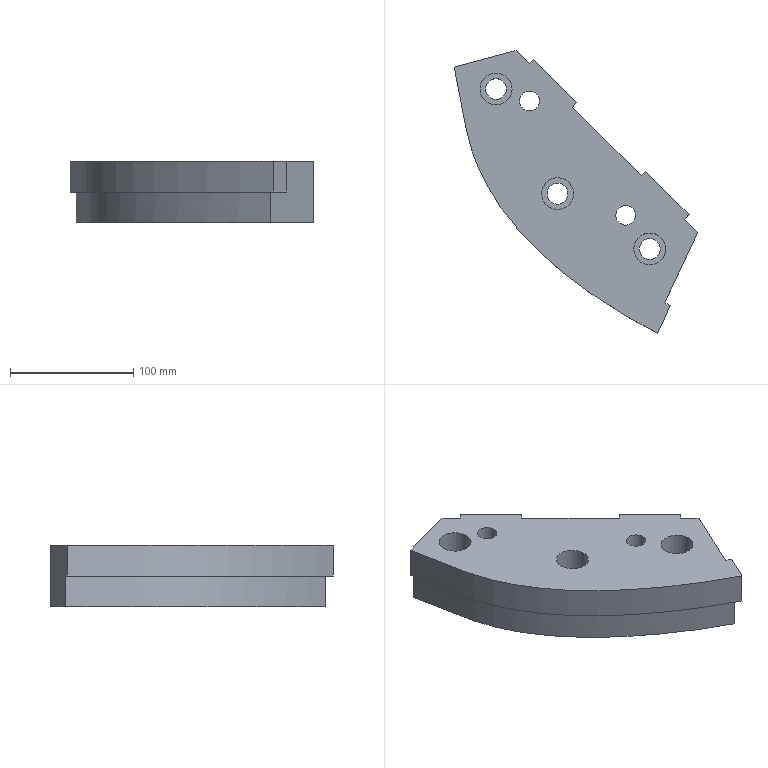Part | NX | features solid 2 | 1 solid | 29 faces | box 197.946 x 229.951 x 50 mm | volume 1003204 mm3 | plane 19 | cylinder 8 | spline 2 | commonest cylinder face diameters 17 x3 26 x3 16 x2
STEP:
#1=CARTESIAN_POINT('',(-617.89,-159.555,-25.));
#2=VERTEX_POINT('',#1);
#3=CARTESIAN_POINT('',(-609.536,-141.638,-25.));
#4=VERTEX_POINT('',#3);
#5=CARTESIAN_POINT('',(-620.101,-164.296,-25.));
#6=DIRECTION('',(-0.4226,-0.9063,0.));
#7=VECTOR('',#6,1000.);
#8=LINE('',#5,#7);
#9=EDGE_CURVE('',#2,#4,#8,.F.);
#10=ORIENTED_EDGE('',*,*,#9,.T.);
#11=CARTESIAN_POINT('',(-605.004,-143.752,-25.));
#12=VERTEX_POINT('',#11);
#13=CARTESIAN_POINT('',(-609.536,-141.638,-25.));
#14=DIRECTION('',(0.9063,-0.4226,0.));
#15=VECTOR('',#14,1000.);
#16=LINE('',#13,#15);
#17=EDGE_CURVE('',#4,#12,#16,.T.);
#18=ORIENTED_EDGE('',*,*,#17,.T.);
#19=CARTESIAN_POINT('',(-615.57,-166.409,-25.));
#20=VERTEX_POINT('',#19);
#21=CARTESIAN_POINT('',(-615.57,-166.409,-25.));
#22=DIRECTION('',(-0.4226,-0.9063,0.));
#23=VECTOR('',#22,1000.);
#24=LINE('',#21,#23);
#25=EDGE_CURVE('',#12,#20,#24,.T.);
#26=ORIENTED_EDGE('',*,*,#25,.T.);
#27=CARTESIAN_POINT('',(-780.695,50.088,-25.));
#28=VERTEX_POINT('',#27);
#29=CARTESIAN_POINT('',(-780.695,50.088,-25.));
#30=CARTESIAN_POINT('',(-778.803,40.269,-25.));
#31=CARTESIAN_POINT('',(-776.28,27.176,-25.));
#32=CARTESIAN_POINT('',(-773.127,10.811,-25.));
#33=CARTESIAN_POINT('',(-771.556,2.503,-25.));
#34=CARTESIAN_POINT('',(-770.053,-4.764,-25.));
#35=CARTESIAN_POINT('',(-768.05,-12.691,-25.));
#36=CARTESIAN_POINT('',(-763.621,-26.574,-25.));
#37=CARTESIAN_POINT('',(-751.782,-52.713,-25.));
#38=CARTESIAN_POINT('',(-727.402,-85.879,-25.));
#39=CARTESIAN_POINT('',(-691.163,-119.147,-25.));
#40=CARTESIAN_POINT('',(-653.334,-145.582,-25.));
#41=CARTESIAN_POINT('',(-627.462,-160.273,-25.));
#42=CARTESIAN_POINT('',(-615.57,-166.409,-25.));
#43=B_SPLINE_CURVE_WITH_KNOTS('',3,(#29,#30,#31,#32,#33,#34,#35,#36,#37,#38,#39,#40,#41,#42),.UNSPECIFIED.,.F.,.F.,(4,1,1,1,1,1,1,1,1,1,1,4),(0.,0.1048,0.1397,0.1746,0.1934,0.2175,0.2603,0.3459,0.5172,0.6885,0.8598,1.),.UNSPECIFIED.);
#44=EDGE_CURVE('',#20,#28,#43,.F.);
#45=ORIENTED_EDGE('',*,*,#44,.T.);
#46=CARTESIAN_POINT('',(-775.853,51.386,-25.));
#47=VERTEX_POINT('',#46);
#48=CARTESIAN_POINT('',(-780.695,50.088,-25.));
#49=DIRECTION('',(-0.9659,-0.2588,0.));
#50=VECTOR('',#49,1000.);
#51=LINE('',#48,#50);
#52=EDGE_CURVE('',#47,#28,#51,.T.);
#53=ORIENTED_EDGE('',*,*,#52,.F.);
#54=CARTESIAN_POINT('',(-775.853,51.386,-25.));
#55=CARTESIAN_POINT('',(-774.744,45.629,-25.));
#56=CARTESIAN_POINT('',(-772.527,34.112,-25.));
#57=CARTESIAN_POINT('',(-769.748,19.729,-25.));
#58=CARTESIAN_POINT('',(-767.541,8.189,-25.));
#59=CARTESIAN_POINT('',(-765.905,-0.4077,-25.));
#60=CARTESIAN_POINT('',(-763.978,-8.633,-25.));
#61=CARTESIAN_POINT('',(-760.703,-19.53,-25.));
#62=CARTESIAN_POINT('',(-755.498,-32.754,-25.));
#63=CARTESIAN_POINT('',(-744.953,-52.969,-25.));
#64=CARTESIAN_POINT('',(-728.152,-76.258,-25.));
#65=CARTESIAN_POINT('',(-703.994,-101.032,-25.));
#66=CARTESIAN_POINT('',(-668.1,-130.302,-25.));
#67=CARTESIAN_POINT('',(-638.408,-148.692,-25.));
#68=CARTESIAN_POINT('',(-617.89,-159.555,-25.));
#69=B_SPLINE_CURVE_WITH_KNOTS('',3,(#54,#55,#56,#57,#58,#59,#60,#61,#62,#63,#64,#65,#66,#67,#68),.UNSPECIFIED.,.F.,.F.,(4,1,1,1,1,1,1,1,1,1,1,1,4),(-0.00125,0.06018,0.1216,0.1523,0.183,0.2138,0.2445,0.3059,0.3673,0.4902,0.6131,0.7359,0.9816),.UNSPECIFIED.);
#70=EDGE_CURVE('',#47,#2,#69,.T.);
#71=ORIENTED_EDGE('',*,*,#70,.T.);
#72=EDGE_LOOP('',(#10,#18,#26,#45,#53,#71));
#73=FACE_BOUND('',#72,.T.);
#74=CARTESIAN_POINT('',(-615.57,-166.409,-25.));
#75=DIRECTION('',(0.,0.,-1.));
#76=DIRECTION('',(-1.,0.,0.));
#77=AXIS2_PLACEMENT_3D('',#74,#75,#76);
#78=PLANE('',#77);
#79=ADVANCED_FACE('',(#73),#78,.T.);
#80=CARTESIAN_POINT('',(-727.523,22.579,0.));
#81=VERTEX_POINT('',#80);
#82=CARTESIAN_POINT('',(-719.523,22.579,0.));
#83=DIRECTION('',(0.,0.,-1.));
#84=DIRECTION('',(-1.,0.,0.));
#85=AXIS2_PLACEMENT_3D('',#82,#83,#84);
#86=CIRCLE('',#85,8.);
#87=EDGE_CURVE('',#81,#81,#86,.T.);
#88=ORIENTED_EDGE('',*,*,#87,.T.);
#89=EDGE_LOOP('',(#88));
#90=FACE_BOUND('',#89,.T.);
#91=CARTESIAN_POINT('',(-649.374,-70.368,0.));
#92=VERTEX_POINT('',#91);
#93=CARTESIAN_POINT('',(-641.374,-70.368,0.));
#94=DIRECTION('',(0.,0.,-1.));
#95=DIRECTION('',(-1.,0.,0.));
#96=AXIS2_PLACEMENT_3D('',#93,#94,#95);
#97=CIRCLE('',#96,8.);
#98=EDGE_CURVE('',#92,#92,#97,.T.);
#99=ORIENTED_EDGE('',*,*,#98,.T.);
#100=EDGE_LOOP('',(#99));
#101=FACE_BOUND('',#100,.T.);
#102=CARTESIAN_POINT('',(-683.729,-52.741,0.));
#103=VERTEX_POINT('',#102);
#104=CARTESIAN_POINT('',(-696.729,-52.741,0.));
#105=DIRECTION('',(0.,0.,1.));
#106=DIRECTION('',(1.,0.,0.));
#107=AXIS2_PLACEMENT_3D('',#104,#105,#106);
#108=CIRCLE('',#107,13.);
#109=EDGE_CURVE('',#103,#103,#108,.T.);
#110=ORIENTED_EDGE('',*,*,#109,.F.);
#111=EDGE_LOOP('',(#110));
#112=FACE_BOUND('',#111,.T.);
#113=CARTESIAN_POINT('',(-608.729,-97.741,0.));
#114=VERTEX_POINT('',#113);
#115=CARTESIAN_POINT('',(-621.729,-97.741,0.));
#116=DIRECTION('',(0.,0.,1.));
#117=DIRECTION('',(1.,0.,0.));
#118=AXIS2_PLACEMENT_3D('',#115,#116,#117);
#119=CIRCLE('',#118,13.);
#120=EDGE_CURVE('',#114,#114,#119,.T.);
#121=ORIENTED_EDGE('',*,*,#120,.F.);
#122=EDGE_LOOP('',(#121));
#123=FACE_BOUND('',#122,.T.);
#124=CARTESIAN_POINT('',(-733.729,32.259,0.));
#125=VERTEX_POINT('',#124);
#126=CARTESIAN_POINT('',(-746.729,32.259,0.));
#127=DIRECTION('',(0.,0.,1.));
#128=DIRECTION('',(1.,0.,0.));
#129=AXIS2_PLACEMENT_3D('',#126,#127,#128);
#130=CIRCLE('',#129,13.);
#131=EDGE_CURVE('',#125,#125,#130,.T.);
#132=ORIENTED_EDGE('',*,*,#131,.F.);
#133=EDGE_LOOP('',(#132));
#134=FACE_BOUND('',#133,.T.);
#135=CARTESIAN_POINT('',(-609.536,-141.638,0.));
#136=VERTEX_POINT('',#135);
#137=CARTESIAN_POINT('',(-605.004,-143.752,0.));
#138=VERTEX_POINT('',#137);
#139=CARTESIAN_POINT('',(-609.536,-141.638,0.));
#140=DIRECTION('',(0.9063,-0.4226,0.));
#141=VECTOR('',#140,1000.);
#142=LINE('',#139,#141);
#143=EDGE_CURVE('',#136,#138,#142,.T.);
#144=ORIENTED_EDGE('',*,*,#143,.F.);
#145=CARTESIAN_POINT('',(-582.749,-84.195,0.));
#146=VERTEX_POINT('',#145);
#147=CARTESIAN_POINT('',(-620.101,-164.296,0.));
#148=DIRECTION('',(0.4226,0.9063,0.));
#149=VECTOR('',#148,1000.);
#150=LINE('',#147,#149);
#151=EDGE_CURVE('',#136,#146,#150,.T.);
#152=ORIENTED_EDGE('',*,*,#151,.T.);
#153=CARTESIAN_POINT('',(-593.356,-73.588,0.));
#154=VERTEX_POINT('',#153);
#155=CARTESIAN_POINT('',(-730.486,63.542,0.));
#156=DIRECTION('',(0.7071,-0.7071,0.));
#157=VECTOR('',#156,1000.);
#158=LINE('',#155,#157);
#159=EDGE_CURVE('',#154,#146,#158,.T.);
#160=ORIENTED_EDGE('',*,*,#159,.F.);
#161=CARTESIAN_POINT('',(-589.82,-70.052,0.));
#162=VERTEX_POINT('',#161);
#163=CARTESIAN_POINT('',(-593.356,-73.588,0.));
#164=DIRECTION('',(0.7071,0.7071,0.));
#165=VECTOR('',#164,1000.);
#166=LINE('',#163,#165);
#167=EDGE_CURVE('',#154,#162,#166,.T.);
#168=ORIENTED_EDGE('',*,*,#167,.T.);
#169=CARTESIAN_POINT('',(-625.176,-34.697,0.));
#170=VERTEX_POINT('',#169);
#171=CARTESIAN_POINT('',(-726.95,67.077,0.));
#172=DIRECTION('',(0.7071,-0.7071,0.));
#173=VECTOR('',#172,1000.);
#174=LINE('',#171,#173);
#175=EDGE_CURVE('',#170,#162,#174,.T.);
#176=ORIENTED_EDGE('',*,*,#175,.F.);
#177=CARTESIAN_POINT('',(-628.711,-38.233,0.));
#178=VERTEX_POINT('',#177);
#179=CARTESIAN_POINT('',(-628.711,-38.233,0.));
#180=DIRECTION('',(0.7071,0.7071,0.));
#181=VECTOR('',#180,1000.);
#182=LINE('',#179,#181);
#183=EDGE_CURVE('',#178,#170,#182,.T.);
#184=ORIENTED_EDGE('',*,*,#183,.F.);
#185=CARTESIAN_POINT('',(-684.524,17.58,0.));
#186=VERTEX_POINT('',#185);
#187=CARTESIAN_POINT('',(-730.486,63.542,0.));
#188=DIRECTION('',(0.7071,-0.7071,0.));
#189=VECTOR('',#188,1000.);
#190=LINE('',#187,#189);
#191=EDGE_CURVE('',#186,#178,#190,.T.);
#192=ORIENTED_EDGE('',*,*,#191,.F.);
#193=CARTESIAN_POINT('',(-680.988,21.115,0.));
#194=VERTEX_POINT('',#193);
#195=CARTESIAN_POINT('',(-684.524,17.58,0.));
#196=DIRECTION('',(0.7071,0.7071,0.));
#197=VECTOR('',#196,1000.);
#198=LINE('',#195,#197);
#199=EDGE_CURVE('',#186,#194,#198,.T.);
#200=ORIENTED_EDGE('',*,*,#199,.T.);
#201=CARTESIAN_POINT('',(-716.343,56.471,0.));
#202=VERTEX_POINT('',#201);
#203=CARTESIAN_POINT('',(-828.725,168.852,0.));
#204=DIRECTION('',(0.7071,-0.7071,0.));
#205=VECTOR('',#204,1000.);
#206=LINE('',#203,#205);
#207=EDGE_CURVE('',#202,#194,#206,.T.);
#208=ORIENTED_EDGE('',*,*,#207,.F.);
#209=CARTESIAN_POINT('',(-719.879,52.935,0.));
#210=VERTEX_POINT('',#209);
#211=CARTESIAN_POINT('',(-719.879,52.935,0.));
#212=DIRECTION('',(0.7071,0.7071,0.));
#213=VECTOR('',#212,1000.);
#214=LINE('',#211,#213);
#215=EDGE_CURVE('',#210,#202,#214,.T.);
#216=ORIENTED_EDGE('',*,*,#215,.F.);
#217=CARTESIAN_POINT('',(-730.486,63.542,0.));
#218=VERTEX_POINT('',#217);
#219=CARTESIAN_POINT('',(-730.486,63.542,0.));
#220=DIRECTION('',(0.7071,-0.7071,0.));
#221=VECTOR('',#220,1000.);
#222=LINE('',#219,#221);
#223=EDGE_CURVE('',#218,#210,#222,.T.);
#224=ORIENTED_EDGE('',*,*,#223,.F.);
#225=CARTESIAN_POINT('',(-780.695,50.088,0.));
#226=VERTEX_POINT('',#225);
#227=CARTESIAN_POINT('',(-780.695,50.088,0.));
#228=DIRECTION('',(0.9659,0.2588,0.));
#229=VECTOR('',#228,1000.);
#230=LINE('',#227,#229);
#231=EDGE_CURVE('',#226,#218,#230,.T.);
#232=ORIENTED_EDGE('',*,*,#231,.F.);
#233=CARTESIAN_POINT('',(-615.57,-166.409,0.));
#234=VERTEX_POINT('',#233);
#235=CARTESIAN_POINT('',(-780.695,50.088,0.));
#236=CARTESIAN_POINT('',(-778.803,40.269,0.));
#237=CARTESIAN_POINT('',(-776.28,27.176,0.));
#238=CARTESIAN_POINT('',(-773.127,10.811,0.));
#239=CARTESIAN_POINT('',(-771.556,2.503,0.));
#240=CARTESIAN_POINT('',(-770.053,-4.764,0.));
#241=CARTESIAN_POINT('',(-768.05,-12.691,0.));
#242=CARTESIAN_POINT('',(-763.621,-26.574,0.));
#243=CARTESIAN_POINT('',(-751.782,-52.713,0.));
#244=CARTESIAN_POINT('',(-727.402,-85.879,0.));
#245=CARTESIAN_POINT('',(-691.163,-119.147,0.));
#246=CARTESIAN_POINT('',(-653.334,-145.582,0.));
#247=CARTESIAN_POINT('',(-627.462,-160.273,0.));
#248=CARTESIAN_POINT('',(-615.57,-166.409,0.));
#249=B_SPLINE_CURVE_WITH_KNOTS('',3,(#235,#236,#237,#238,#239,#240,#241,#242,#243,#244,#245,#246,#247,#248),.UNSPECIFIED.,.F.,.F.,(4,1,1,1,1,1,1,1,1,1,1,4),(0.,0.1048,0.1397,0.1746,0.1934,0.2175,0.2603,0.3459,0.5172,0.6885,0.8598,1.),.UNSPECIFIED.);
#250=EDGE_CURVE('',#226,#234,#249,.T.);
#251=ORIENTED_EDGE('',*,*,#250,.T.);
#252=CARTESIAN_POINT('',(-615.57,-166.409,0.));
#253=DIRECTION('',(0.4226,0.9063,0.));
#254=VECTOR('',#253,1000.);
#255=LINE('',#252,#254);
#256=EDGE_CURVE('',#234,#138,#255,.T.);
#257=ORIENTED_EDGE('',*,*,#256,.T.);
#258=EDGE_LOOP('',(#144,#152,#160,#168,#176,#184,#192,#200,#208,#216,#224,#232,#251,#257));
#259=FACE_BOUND('',#258,.T.);
#260=CARTESIAN_POINT('',(-733.42,73.248,0.));
#261=DIRECTION('',(0.,0.,-1.));
#262=DIRECTION('',(-1.,0.,0.));
#263=AXIS2_PLACEMENT_3D('',#260,#261,#262);
#264=PLANE('',#263);
#265=ADVANCED_FACE('',(#90,#101,#112,#123,#134,#259),#264,.F.);
#266=ORIENTED_EDGE('',*,*,#25,.F.);
#267=CARTESIAN_POINT('',(-605.004,-143.752,-50.));
#268=DIRECTION('',(0.,0.,1.));
#269=VECTOR('',#268,1000.);
#270=LINE('',#267,#269);
#271=EDGE_CURVE('',#12,#138,#270,.T.);
#272=ORIENTED_EDGE('',*,*,#271,.T.);
#273=ORIENTED_EDGE('',*,*,#256,.F.);
#274=CARTESIAN_POINT('',(-615.57,-166.409,-70.));
#275=DIRECTION('',(0.,0.,1.));
#276=VECTOR('',#275,1000.);
#277=LINE('',#274,#276);
#278=EDGE_CURVE('',#20,#234,#277,.T.);
#279=ORIENTED_EDGE('',*,*,#278,.F.);
#280=EDGE_LOOP('',(#266,#272,#273,#279));
#281=FACE_BOUND('',#280,.T.);
#282=CARTESIAN_POINT('',(-615.57,-166.409,-50.));
#283=DIRECTION('',(0.9063,-0.4226,0.));
#284=DIRECTION('',(0.4226,0.9063,0.));
#285=AXIS2_PLACEMENT_3D('',#282,#283,#284);
#286=PLANE('',#285);
#287=ADVANCED_FACE('',(#281),#286,.T.);
#288=ORIENTED_EDGE('',*,*,#159,.T.);
#289=CARTESIAN_POINT('',(-582.749,-84.195,-50.));
#290=VERTEX_POINT('',#289);
#291=CARTESIAN_POINT('',(-582.749,-84.195,-50.));
#292=DIRECTION('',(0.,0.,-1.));
#293=VECTOR('',#292,1000.);
#294=LINE('',#291,#293);
#295=EDGE_CURVE('',#146,#290,#294,.T.);
#296=ORIENTED_EDGE('',*,*,#295,.T.);
#297=CARTESIAN_POINT('',(-593.356,-73.588,-50.));
#298=VERTEX_POINT('',#297);
#299=CARTESIAN_POINT('',(-730.486,63.542,-50.));
#300=DIRECTION('',(0.7071,-0.7071,0.));
#301=VECTOR('',#300,1000.);
#302=LINE('',#299,#301);
#303=EDGE_CURVE('',#298,#290,#302,.T.);
#304=ORIENTED_EDGE('',*,*,#303,.F.);
#305=CARTESIAN_POINT('',(-593.356,-73.588,-50.));
#306=DIRECTION('',(0.,0.,1.));
#307=VECTOR('',#306,1000.);
#308=LINE('',#305,#307);
#309=EDGE_CURVE('',#298,#154,#308,.T.);
#310=ORIENTED_EDGE('',*,*,#309,.T.);
#311=EDGE_LOOP('',(#288,#296,#304,#310));
#312=FACE_BOUND('',#311,.T.);
#313=CARTESIAN_POINT('',(-730.486,63.542,-50.));
#314=DIRECTION('',(-0.7071,-0.7071,0.));
#315=DIRECTION('',(0.7071,-0.7071,0.));
#316=AXIS2_PLACEMENT_3D('',#313,#314,#315);
#317=PLANE('',#316);
#318=ADVANCED_FACE('',(#312),#317,.F.);
#319=CARTESIAN_POINT('',(-711.523,22.579,-50.));
#320=VERTEX_POINT('',#319);
#321=CARTESIAN_POINT('',(-719.523,22.579,-50.));
#322=DIRECTION('',(0.,0.,1.));
#323=DIRECTION('',(1.,0.,0.));
#324=AXIS2_PLACEMENT_3D('',#321,#322,#323);
#325=CIRCLE('',#324,8.);
#326=EDGE_CURVE('',#320,#320,#325,.T.);
#327=ORIENTED_EDGE('',*,*,#326,.T.);
#328=EDGE_LOOP('',(#327));
#329=FACE_BOUND('',#328,.T.);
#330=CARTESIAN_POINT('',(-633.374,-70.368,-50.));
#331=VERTEX_POINT('',#330);
#332=CARTESIAN_POINT('',(-641.374,-70.368,-50.));
#333=DIRECTION('',(0.,0.,1.));
#334=DIRECTION('',(1.,0.,0.));
#335=AXIS2_PLACEMENT_3D('',#332,#333,#334);
#336=CIRCLE('',#335,8.);
#337=EDGE_CURVE('',#331,#331,#336,.T.);
#338=ORIENTED_EDGE('',*,*,#337,.T.);
#339=EDGE_LOOP('',(#338));
#340=FACE_BOUND('',#339,.T.);
#341=CARTESIAN_POINT('',(-617.89,-159.555,-50.));
#342=VERTEX_POINT('',#341);
#343=CARTESIAN_POINT('',(-607.768,-137.848,-50.));
#344=DIRECTION('',(-0.4226,-0.9063,0.));
#345=VECTOR('',#344,1000.);
#346=LINE('',#343,#345);
#347=EDGE_CURVE('',#290,#342,#346,.T.);
#348=ORIENTED_EDGE('',*,*,#347,.T.);
#349=CARTESIAN_POINT('',(-775.853,51.386,-50.));
#350=VERTEX_POINT('',#349);
#351=CARTESIAN_POINT('',(-617.89,-159.555,-50.));
#352=CARTESIAN_POINT('',(-622.998,-156.85,-50.));
#353=CARTESIAN_POINT('',(-630.561,-152.674,-50.));
#354=CARTESIAN_POINT('',(-639.19,-147.603,-50.));
#355=CARTESIAN_POINT('',(-644.088,-144.635,-50.));
#356=CARTESIAN_POINT('',(-647.684,-142.412,-50.));
#357=CARTESIAN_POINT('',(-651.449,-140.037,-50.));
#358=CARTESIAN_POINT('',(-656.324,-136.895,-50.));
#359=CARTESIAN_POINT('',(-662.31,-132.912,-50.));
#360=CARTESIAN_POINT('',(-668.126,-128.871,-50.));
#361=CARTESIAN_POINT('',(-672.085,-126.03,-50.));
#362=CARTESIAN_POINT('',(-674.358,-124.372,-50.));
#363=CARTESIAN_POINT('',(-675.947,-123.2,-50.));
#364=CARTESIAN_POINT('',(-677.912,-121.734,-50.));
#365=CARTESIAN_POINT('',(-680.368,-119.877,-50.));
#366=CARTESIAN_POINT('',(-683.437,-117.514,-50.));
#367=CARTESIAN_POINT('',(-687.023,-114.68,-50.));
#368=CARTESIAN_POINT('',(-691.708,-110.88,-50.));
#369=CARTESIAN_POINT('',(-697.371,-106.101,-50.));
#370=CARTESIAN_POINT('',(-703.86,-100.315,-50.));
#371=CARTESIAN_POINT('',(-710.042,-94.48,-50.));
#372=CARTESIAN_POINT('',(-714.937,-89.576,-50.));
#373=CARTESIAN_POINT('',(-718.7,-85.627,-50.));
#374=CARTESIAN_POINT('',(-721.444,-82.656,-50.));
#375=CARTESIAN_POINT('',(-723.673,-80.162,-50.));
#376=CARTESIAN_POINT('',(-725.186,-78.425,-50.));
#377=CARTESIAN_POINT('',(-726.062,-77.408,-50.));
#378=CARTESIAN_POINT('',(-726.657,-76.711,-50.));
#379=CARTESIAN_POINT('',(-727.462,-75.759,-50.));
#380=CARTESIAN_POINT('',(-728.451,-74.577,-50.));
#381=CARTESIAN_POINT('',(-730.192,-72.464,-50.));
#382=CARTESIAN_POINT('',(-732.591,-69.456,-50.));
#383=CARTESIAN_POINT('',(-735.368,-65.82,-50.));
#384=CARTESIAN_POINT('',(-738.921,-60.952,-50.));
#385=CARTESIAN_POINT('',(-743.087,-54.822,-50.));
#386=CARTESIAN_POINT('',(-749.161,-44.924,-50.));
#387=CARTESIAN_POINT('',(-754.356,-34.877,-50.));
#388=CARTESIAN_POINT('',(-758.119,-25.991,-50.));
#389=CARTESIAN_POINT('',(-760.062,-20.837,-50.));
#390=CARTESIAN_POINT('',(-761.372,-17.07,-50.));
#391=CARTESIAN_POINT('',(-762.709,-12.844,-50.));
#392=CARTESIAN_POINT('',(-763.892,-8.672,-50.));
#393=CARTESIAN_POINT('',(-764.791,-5.118,-50.));
#394=CARTESIAN_POINT('',(-765.365,-2.621,-50.));
#395=CARTESIAN_POINT('',(-765.643,-1.351,-50.));
#396=CARTESIAN_POINT('',(-765.793,-0.6486,-50.));
#397=CARTESIAN_POINT('',(-765.918,-0.04992,-50.));
#398=CARTESIAN_POINT('',(-765.986,0.2783,-50.));
#399=CARTESIAN_POINT('',(-766.102,0.8432,-50.));
#400=CARTESIAN_POINT('',(-766.307,1.853,-50.));
#401=CARTESIAN_POINT('',(-766.637,3.514,-50.));
#402=CARTESIAN_POINT('',(-767.013,5.436,-50.));
#403=CARTESIAN_POINT('',(-767.295,6.9,-50.));
#404=CARTESIAN_POINT('',(-767.469,7.808,-50.));
#405=CARTESIAN_POINT('',(-767.586,8.417,-50.));
#406=CARTESIAN_POINT('',(-767.772,9.392,-50.));
#407=CARTESIAN_POINT('',(-767.982,10.486,-50.));
#408=CARTESIAN_POINT('',(-768.23,11.784,-50.));
#409=CARTESIAN_POINT('',(-768.488,13.135,-50.));
#410=CARTESIAN_POINT('',(-768.786,14.69,-50.));
#411=CARTESIAN_POINT('',(-769.014,15.883,-50.));
#412=CARTESIAN_POINT('',(-769.162,16.657,-50.));
#413=CARTESIAN_POINT('',(-769.244,17.082,-50.));
#414=CARTESIAN_POINT('',(-769.249,17.106,-50.));
#415=CARTESIAN_POINT('',(-769.269,17.211,-50.));
#416=CARTESIAN_POINT('',(-769.309,17.421,-50.));
#417=CARTESIAN_POINT('',(-769.399,17.887,-50.));
#418=CARTESIAN_POINT('',(-769.553,18.686,-50.));
#419=CARTESIAN_POINT('',(-769.821,20.079,-50.));
#420=CARTESIAN_POINT('',(-770.274,22.431,-50.));
#421=CARTESIAN_POINT('',(-771.007,26.232,-50.));
#422=CARTESIAN_POINT('',(-771.927,31.012,-50.));
#423=CARTESIAN_POINT('',(-773.407,38.69,-50.));
#424=CARTESIAN_POINT('',(-774.799,45.916,-50.));
#425=CARTESIAN_POINT('',(-775.853,51.386,-50.));
#426=B_SPLINE_CURVE_WITH_KNOTS('',3,(#351,#352,#353,#354,#355,#356,#357,#358,#359,#360,#361,#362,#363,#364,#365,#366,#367,#368,#369,#370,#371,#372,#373,#374,#375,#376,#377,#378,#379,#380,#381,#382,#383,#384,#385,#386,#387,#388,#389,#390,#391,#392,#393,#394,#395,#396,#397,#398,#399,#400,#401,#402,#403,#404,#405,#406,#407,#408,#409,#410,#411,#412,#413,#414,#415,#416,#417,#418,#419,#420,#421,#422,#423,#424,#425),.UNSPECIFIED.,.F.,.F.,(4,1,1,1,1,1,1,1,1,1,1,1,1,1,1,1,1,1,1,1,1,1,1,1,1,1,1,1,1,1,1,1,1,1,1,1,1,1,1,1,1,1,1,1,1,1,1,1,1,1,1,1,1,1,1,1,1,1,1,1,1,1,1,1,1,1,1,1,1,1,1,1,4),(0.,0.0625,0.09375,0.1094,0.125,0.1406,0.1562,0.1875,0.2188,0.2344,0.2422,0.25,0.2578,0.2656,0.2812,0.2969,0.3125,0.3438,0.375,0.4062,0.4375,0.4531,0.4688,0.4844,0.4922,0.4961,0.5,0.5039,0.5078,0.5156,0.5312,0.5469,0.5625,0.5938,0.625,0.6875,0.7188,0.7344,0.75,0.7656,0.7812,0.7969,0.8047,0.8086,0.8105,0.8125,0.8145,0.8164,0.8203,0.8281,0.8359,0.8398,0.8418,0.8438,0.8457,0.8477,0.8516,0.8555,0.8594,0.8672,0.8711,0.875,0.877,0.8789,0.8828,0.8906,0.8984,0.9062,0.9219,0.9375,0.9531,0.9688,1.),.UNSPECIFIED.);
#427=EDGE_CURVE('',#342,#350,#426,.T.);
#428=ORIENTED_EDGE('',*,*,#427,.T.);
#429=CARTESIAN_POINT('',(-730.486,63.542,-50.));
#430=VERTEX_POINT('',#429);
#431=CARTESIAN_POINT('',(-780.695,50.088,-50.));
#432=DIRECTION('',(0.9659,0.2588,0.));
#433=VECTOR('',#432,1000.);
#434=LINE('',#431,#433);
#435=EDGE_CURVE('',#350,#430,#434,.T.);
#436=ORIENTED_EDGE('',*,*,#435,.T.);
#437=CARTESIAN_POINT('',(-719.879,52.935,-50.));
#438=VERTEX_POINT('',#437);
#439=CARTESIAN_POINT('',(-730.486,63.542,-50.));
#440=DIRECTION('',(0.7071,-0.7071,0.));
#441=VECTOR('',#440,1000.);
#442=LINE('',#439,#441);
#443=EDGE_CURVE('',#430,#438,#442,.T.);
#444=ORIENTED_EDGE('',*,*,#443,.T.);
#445=CARTESIAN_POINT('',(-716.343,56.471,-50.));
#446=VERTEX_POINT('',#445);
#447=CARTESIAN_POINT('',(-719.879,52.935,-50.));
#448=DIRECTION('',(0.7071,0.7071,0.));
#449=VECTOR('',#448,1000.);
#450=LINE('',#447,#449);
#451=EDGE_CURVE('',#438,#446,#450,.T.);
#452=ORIENTED_EDGE('',*,*,#451,.T.);
#453=CARTESIAN_POINT('',(-680.988,21.115,-50.));
#454=VERTEX_POINT('',#453);
#455=CARTESIAN_POINT('',(-828.725,168.852,-50.));
#456=DIRECTION('',(0.7071,-0.7071,0.));
#457=VECTOR('',#456,1000.);
#458=LINE('',#455,#457);
#459=EDGE_CURVE('',#446,#454,#458,.T.);
#460=ORIENTED_EDGE('',*,*,#459,.T.);
#461=CARTESIAN_POINT('',(-684.524,17.58,-50.));
#462=VERTEX_POINT('',#461);
#463=CARTESIAN_POINT('',(-684.524,17.58,-50.));
#464=DIRECTION('',(0.7071,0.7071,0.));
#465=VECTOR('',#464,1000.);
#466=LINE('',#463,#465);
#467=EDGE_CURVE('',#462,#454,#466,.T.);
#468=ORIENTED_EDGE('',*,*,#467,.F.);
#469=CARTESIAN_POINT('',(-628.711,-38.233,-50.));
#470=VERTEX_POINT('',#469);
#471=CARTESIAN_POINT('',(-730.486,63.542,-50.));
#472=DIRECTION('',(0.7071,-0.7071,0.));
#473=VECTOR('',#472,1000.);
#474=LINE('',#471,#473);
#475=EDGE_CURVE('',#462,#470,#474,.T.);
#476=ORIENTED_EDGE('',*,*,#475,.T.);
#477=CARTESIAN_POINT('',(-625.176,-34.697,-50.));
#478=VERTEX_POINT('',#477);
#479=CARTESIAN_POINT('',(-628.711,-38.233,-50.));
#480=DIRECTION('',(0.7071,0.7071,0.));
#481=VECTOR('',#480,1000.);
#482=LINE('',#479,#481);
#483=EDGE_CURVE('',#470,#478,#482,.T.);
#484=ORIENTED_EDGE('',*,*,#483,.T.);
#485=CARTESIAN_POINT('',(-589.82,-70.052,-50.));
#486=VERTEX_POINT('',#485);
#487=CARTESIAN_POINT('',(-726.95,67.077,-50.));
#488=DIRECTION('',(0.7071,-0.7071,0.));
#489=VECTOR('',#488,1000.);
#490=LINE('',#487,#489);
#491=EDGE_CURVE('',#478,#486,#490,.T.);
#492=ORIENTED_EDGE('',*,*,#491,.T.);
#493=CARTESIAN_POINT('',(-593.356,-73.588,-50.));
#494=DIRECTION('',(0.7071,0.7071,0.));
#495=VECTOR('',#494,1000.);
#496=LINE('',#493,#495);
#497=EDGE_CURVE('',#298,#486,#496,.T.);
#498=ORIENTED_EDGE('',*,*,#497,.F.);
#499=ORIENTED_EDGE('',*,*,#303,.T.);
#500=EDGE_LOOP('',(#348,#428,#436,#444,#452,#460,#468,#476,#484,#492,#498,#499));
#501=FACE_BOUND('',#500,.T.);
#502=CARTESIAN_POINT('',(-613.229,-97.741,-50.));
#503=VERTEX_POINT('',#502);
#504=CARTESIAN_POINT('',(-621.729,-97.741,-50.));
#505=DIRECTION('',(0.,0.,1.));
#506=DIRECTION('',(1.,0.,0.));
#507=AXIS2_PLACEMENT_3D('',#504,#505,#506);
#508=CIRCLE('',#507,8.5);
#509=EDGE_CURVE('',#503,#503,#508,.T.);
#510=ORIENTED_EDGE('',*,*,#509,.T.);
#511=EDGE_LOOP('',(#510));
#512=FACE_BOUND('',#511,.T.);
#513=CARTESIAN_POINT('',(-738.229,32.259,-50.));
#514=VERTEX_POINT('',#513);
#515=CARTESIAN_POINT('',(-746.729,32.259,-50.));
#516=DIRECTION('',(0.,0.,1.));
#517=DIRECTION('',(1.,0.,0.));
#518=AXIS2_PLACEMENT_3D('',#515,#516,#517);
#519=CIRCLE('',#518,8.5);
#520=EDGE_CURVE('',#514,#514,#519,.T.);
#521=ORIENTED_EDGE('',*,*,#520,.T.);
#522=EDGE_LOOP('',(#521));
#523=FACE_BOUND('',#522,.T.);
#524=CARTESIAN_POINT('',(-688.229,-52.741,-50.));
#525=VERTEX_POINT('',#524);
#526=CARTESIAN_POINT('',(-696.729,-52.741,-50.));
#527=DIRECTION('',(0.,0.,1.));
#528=DIRECTION('',(1.,0.,0.));
#529=AXIS2_PLACEMENT_3D('',#526,#527,#528);
#530=CIRCLE('',#529,8.5);
#531=EDGE_CURVE('',#525,#525,#530,.T.);
#532=ORIENTED_EDGE('',*,*,#531,.T.);
#533=EDGE_LOOP('',(#532));
#534=FACE_BOUND('',#533,.T.);
#535=CARTESIAN_POINT('',(-927.359,-581.717,-50.));
#536=DIRECTION('',(0.,0.,1.));
#537=DIRECTION('',(1.,0.,0.));
#538=AXIS2_PLACEMENT_3D('',#535,#536,#537);
#539=PLANE('',#538);
#540=ADVANCED_FACE('',(#329,#340,#501,#512,#523,#534),#539,.F.);
#541=ORIENTED_EDGE('',*,*,#120,.T.);
#542=EDGE_LOOP('',(#541));
#543=FACE_BOUND('',#542,.T.);
#544=CARTESIAN_POINT('',(-608.729,-97.741,-25.));
#545=VERTEX_POINT('',#544);
#546=CARTESIAN_POINT('',(-621.729,-97.741,-25.));
#547=DIRECTION('',(0.,0.,1.));
#548=DIRECTION('',(1.,0.,0.));
#549=AXIS2_PLACEMENT_3D('',#546,#547,#548);
#550=CIRCLE('',#549,13.);
#551=EDGE_CURVE('',#545,#545,#550,.T.);
#552=ORIENTED_EDGE('',*,*,#551,.F.);
#553=EDGE_LOOP('',(#552));
#554=FACE_BOUND('',#553,.T.);
#555=CARTESIAN_POINT('',(-621.729,-97.741,-25.));
#556=DIRECTION('',(0.,0.,1.));
#557=DIRECTION('',(1.,0.,0.));
#558=AXIS2_PLACEMENT_3D('',#555,#556,#557);
#559=CYLINDRICAL_SURFACE('',#558,13.);
#560=ADVANCED_FACE('',(#543,#554),#559,.F.);
#561=CARTESIAN_POINT('',(-630.229,-97.741,-25.));
#562=VERTEX_POINT('',#561);
#563=CARTESIAN_POINT('',(-621.729,-97.741,-25.));
#564=DIRECTION('',(0.,0.,-1.));
#565=DIRECTION('',(-1.,0.,0.));
#566=AXIS2_PLACEMENT_3D('',#563,#564,#565);
#567=CIRCLE('',#566,8.5);
#568=EDGE_CURVE('',#562,#562,#567,.F.);
#569=ORIENTED_EDGE('',*,*,#568,.T.);
#570=EDGE_LOOP('',(#569));
#571=FACE_BOUND('',#570,.T.);
#572=ORIENTED_EDGE('',*,*,#509,.F.);
#573=EDGE_LOOP('',(#572));
#574=FACE_BOUND('',#573,.T.);
#575=CARTESIAN_POINT('',(-621.729,-97.741,-75.));
#576=DIRECTION('',(0.,0.,1.));
#577=DIRECTION('',(1.,0.,0.));
#578=AXIS2_PLACEMENT_3D('',#575,#576,#577);
#579=CYLINDRICAL_SURFACE('',#578,8.5);
#580=ADVANCED_FACE('',(#571,#574),#579,.F.);
#581=ORIENTED_EDGE('',*,*,#568,.F.);
#582=EDGE_LOOP('',(#581));
#583=FACE_BOUND('',#582,.T.);
#584=ORIENTED_EDGE('',*,*,#551,.T.);
#585=EDGE_LOOP('',(#584));
#586=FACE_BOUND('',#585,.T.);
#587=CARTESIAN_POINT('',(-621.729,-97.741,-25.));
#588=DIRECTION('',(0.,0.,-1.));
#589=DIRECTION('',(-1.,0.,0.));
#590=AXIS2_PLACEMENT_3D('',#587,#588,#589);
#591=PLANE('',#590);
#592=ADVANCED_FACE('',(#583,#586),#591,.F.);
#593=ORIENTED_EDGE('',*,*,#531,.F.);
#594=EDGE_LOOP('',(#593));
#595=FACE_BOUND('',#594,.T.);
#596=CARTESIAN_POINT('',(-705.229,-52.741,-25.));
#597=VERTEX_POINT('',#596);
#598=CARTESIAN_POINT('',(-696.729,-52.741,-25.));
#599=DIRECTION('',(0.,0.,-1.));
#600=DIRECTION('',(-1.,0.,0.));
#601=AXIS2_PLACEMENT_3D('',#598,#599,#600);
#602=CIRCLE('',#601,8.5);
#603=EDGE_CURVE('',#597,#597,#602,.F.);
#604=ORIENTED_EDGE('',*,*,#603,.T.);
#605=EDGE_LOOP('',(#604));
#606=FACE_BOUND('',#605,.T.);
#607=CARTESIAN_POINT('',(-696.729,-52.741,-75.));
#608=DIRECTION('',(0.,0.,1.));
#609=DIRECTION('',(1.,0.,0.));
#610=AXIS2_PLACEMENT_3D('',#607,#608,#609);
#611=CYLINDRICAL_SURFACE('',#610,8.5);
#612=ADVANCED_FACE('',(#595,#606),#611,.F.);
#613=CARTESIAN_POINT('',(-683.729,-52.741,-25.));
#614=VERTEX_POINT('',#613);
#615=CARTESIAN_POINT('',(-696.729,-52.741,-25.));
#616=DIRECTION('',(0.,0.,1.));
#617=DIRECTION('',(1.,0.,0.));
#618=AXIS2_PLACEMENT_3D('',#615,#616,#617);
#619=CIRCLE('',#618,13.);
#620=EDGE_CURVE('',#614,#614,#619,.T.);
#621=ORIENTED_EDGE('',*,*,#620,.F.);
#622=EDGE_LOOP('',(#621));
#623=FACE_BOUND('',#622,.T.);
#624=ORIENTED_EDGE('',*,*,#109,.T.);
#625=EDGE_LOOP('',(#624));
#626=FACE_BOUND('',#625,.T.);
#627=CARTESIAN_POINT('',(-696.729,-52.741,-25.));
#628=DIRECTION('',(0.,0.,1.));
#629=DIRECTION('',(1.,0.,0.));
#630=AXIS2_PLACEMENT_3D('',#627,#628,#629);
#631=CYLINDRICAL_SURFACE('',#630,13.);
#632=ADVANCED_FACE('',(#623,#626),#631,.F.);
#633=ORIENTED_EDGE('',*,*,#603,.F.);
#634=EDGE_LOOP('',(#633));
#635=FACE_BOUND('',#634,.T.);
#636=ORIENTED_EDGE('',*,*,#620,.T.);
#637=EDGE_LOOP('',(#636));
#638=FACE_BOUND('',#637,.T.);
#639=CARTESIAN_POINT('',(-696.729,-52.741,-25.));
#640=DIRECTION('',(0.,0.,-1.));
#641=DIRECTION('',(-1.,0.,0.));
#642=AXIS2_PLACEMENT_3D('',#639,#640,#641);
#643=PLANE('',#642);
#644=ADVANCED_FACE('',(#635,#638),#643,.F.);
#645=CARTESIAN_POINT('',(-755.229,32.259,-25.));
#646=VERTEX_POINT('',#645);
#647=CARTESIAN_POINT('',(-746.729,32.259,-25.));
#648=DIRECTION('',(0.,0.,-1.));
#649=DIRECTION('',(-1.,0.,0.));
#650=AXIS2_PLACEMENT_3D('',#647,#648,#649);
#651=CIRCLE('',#650,8.5);
#652=EDGE_CURVE('',#646,#646,#651,.F.);
#653=ORIENTED_EDGE('',*,*,#652,.T.);
#654=EDGE_LOOP('',(#653));
#655=FACE_BOUND('',#654,.T.);
#656=ORIENTED_EDGE('',*,*,#520,.F.);
#657=EDGE_LOOP('',(#656));
#658=FACE_BOUND('',#657,.T.);
#659=CARTESIAN_POINT('',(-746.729,32.259,-75.));
#660=DIRECTION('',(0.,0.,1.));
#661=DIRECTION('',(1.,0.,0.));
#662=AXIS2_PLACEMENT_3D('',#659,#660,#661);
#663=CYLINDRICAL_SURFACE('',#662,8.5);
#664=ADVANCED_FACE('',(#655,#658),#663,.F.);
#665=CARTESIAN_POINT('',(-733.729,32.259,-25.));
#666=VERTEX_POINT('',#665);
#667=CARTESIAN_POINT('',(-746.729,32.259,-25.));
#668=DIRECTION('',(0.,0.,1.));
#669=DIRECTION('',(1.,0.,0.));
#670=AXIS2_PLACEMENT_3D('',#667,#668,#669);
#671=CIRCLE('',#670,13.);
#672=EDGE_CURVE('',#666,#666,#671,.T.);
#673=ORIENTED_EDGE('',*,*,#672,.F.);
#674=EDGE_LOOP('',(#673));
#675=FACE_BOUND('',#674,.T.);
#676=ORIENTED_EDGE('',*,*,#131,.T.);
#677=EDGE_LOOP('',(#676));
#678=FACE_BOUND('',#677,.T.);
#679=CARTESIAN_POINT('',(-746.729,32.259,-25.));
#680=DIRECTION('',(0.,0.,1.));
#681=DIRECTION('',(1.,0.,0.));
#682=AXIS2_PLACEMENT_3D('',#679,#680,#681);
#683=CYLINDRICAL_SURFACE('',#682,13.);
#684=ADVANCED_FACE('',(#675,#678),#683,.F.);
#685=ORIENTED_EDGE('',*,*,#652,.F.);
#686=EDGE_LOOP('',(#685));
#687=FACE_BOUND('',#686,.T.);
#688=ORIENTED_EDGE('',*,*,#672,.T.);
#689=EDGE_LOOP('',(#688));
#690=FACE_BOUND('',#689,.T.);
#691=CARTESIAN_POINT('',(-746.729,32.259,-25.));
#692=DIRECTION('',(0.,0.,-1.));
#693=DIRECTION('',(-1.,0.,0.));
#694=AXIS2_PLACEMENT_3D('',#691,#692,#693);
#695=PLANE('',#694);
#696=ADVANCED_FACE('',(#687,#690),#695,.F.);
#697=ORIENTED_EDGE('',*,*,#231,.T.);
#698=CARTESIAN_POINT('',(-730.486,63.542,-50.));
#699=DIRECTION('',(0.,0.,1.));
#700=VECTOR('',#699,1000.);
#701=LINE('',#698,#700);
#702=EDGE_CURVE('',#430,#218,#701,.T.);
#703=ORIENTED_EDGE('',*,*,#702,.F.);
#704=ORIENTED_EDGE('',*,*,#435,.F.);
#705=CARTESIAN_POINT('',(-775.853,51.386,-42.5));
#706=DIRECTION('',(0.,0.,-1.));
#707=VECTOR('',#706,1000.);
#708=LINE('',#705,#707);
#709=EDGE_CURVE('',#350,#47,#708,.F.);
#710=ORIENTED_EDGE('',*,*,#709,.T.);
#711=ORIENTED_EDGE('',*,*,#52,.T.);
#712=CARTESIAN_POINT('',(-780.695,50.088,-50.));
#713=DIRECTION('',(0.,0.,1.));
#714=VECTOR('',#713,1000.);
#715=LINE('',#712,#714);
#716=EDGE_CURVE('',#28,#226,#715,.T.);
#717=ORIENTED_EDGE('',*,*,#716,.T.);
#718=EDGE_LOOP('',(#697,#703,#704,#710,#711,#717));
#719=FACE_BOUND('',#718,.T.);
#720=CARTESIAN_POINT('',(-780.695,50.088,-50.));
#721=DIRECTION('',(0.2588,-0.9659,0.));
#722=DIRECTION('',(0.9659,0.2588,0.));
#723=AXIS2_PLACEMENT_3D('',#720,#721,#722);
#724=PLANE('',#723);
#725=ADVANCED_FACE('',(#719),#724,.F.);
#726=ORIENTED_EDGE('',*,*,#44,.F.);
#727=ORIENTED_EDGE('',*,*,#278,.T.);
#728=ORIENTED_EDGE('',*,*,#250,.F.);
#729=ORIENTED_EDGE('',*,*,#716,.F.);
#730=EDGE_LOOP('',(#726,#727,#728,#729));
#731=FACE_BOUND('',#730,.T.);
#732=CARTESIAN_POINT('',(-780.695,50.088,-25.));
#733=CARTESIAN_POINT('',(-780.695,50.088,0.));
#734=CARTESIAN_POINT('',(-779.566,44.231,-25.));
#735=CARTESIAN_POINT('',(-779.566,44.231,0.));
#736=CARTESIAN_POINT('',(-777.312,32.516,-25.));
#737=CARTESIAN_POINT('',(-777.312,32.516,0.));
#738=CARTESIAN_POINT('',(-774.482,17.874,-25.));
#739=CARTESIAN_POINT('',(-774.482,17.874,0.));
#740=CARTESIAN_POINT('',(-772.245,6.156,-25.));
#741=CARTESIAN_POINT('',(-772.245,6.156,0.));
#742=CARTESIAN_POINT('',(-770.561,-2.633,-25.));
#743=CARTESIAN_POINT('',(-770.561,-2.633,0.));
#744=CARTESIAN_POINT('',(-768.427,-11.326,-25.));
#745=CARTESIAN_POINT('',(-768.427,-11.326,0.));
#746=CARTESIAN_POINT('',(-764.886,-22.725,-25.));
#747=CARTESIAN_POINT('',(-764.886,-22.725,0.));
#748=CARTESIAN_POINT('',(-759.263,-36.564,-25.));
#749=CARTESIAN_POINT('',(-759.263,-36.564,0.));
#750=CARTESIAN_POINT('',(-747.969,-57.602,-25.));
#751=CARTESIAN_POINT('',(-747.969,-57.602,0.));
#752=CARTESIAN_POINT('',(-730.151,-81.671,-25.));
#753=CARTESIAN_POINT('',(-730.151,-81.671,0.));
#754=CARTESIAN_POINT('',(-704.817,-107.049,-25.));
#755=CARTESIAN_POINT('',(-704.817,-107.049,0.));
#756=CARTESIAN_POINT('',(-667.472,-136.861,-25.));
#757=CARTESIAN_POINT('',(-667.472,-136.861,0.));
#758=CARTESIAN_POINT('',(-636.774,-155.468,-25.));
#759=CARTESIAN_POINT('',(-636.774,-155.468,0.));
#760=CARTESIAN_POINT('',(-615.57,-166.409,-25.));
#761=CARTESIAN_POINT('',(-615.57,-166.409,0.));
#762=B_SPLINE_SURFACE_WITH_KNOTS('',3,1,((#732,#733),(#734,#735),(#736,#737),(#738,#739),(#740,#741),(#742,#743),(#744,#745),(#746,#747),(#748,#749),(#750,#751),(#752,#753),(#754,#755),(#756,#757),(#758,#759),(#760,#761)),.SURF_OF_LINEAR_EXTRUSION.,.F.,.F.,.F.,(4,1,1,1,1,1,1,1,1,1,1,1,4),(2,2),(0.,0.0625,0.125,0.1562,0.1875,0.2188,0.25,0.3125,0.375,0.5,0.625,0.75,1.),(0.,1.),.UNSPECIFIED.);
#763=ADVANCED_FACE('',(#731),#762,.T.);
#764=ORIENTED_EDGE('',*,*,#70,.F.);
#765=ORIENTED_EDGE('',*,*,#709,.F.);
#766=ORIENTED_EDGE('',*,*,#427,.F.);
#767=CARTESIAN_POINT('',(-617.89,-159.555,-37.5));
#768=DIRECTION('',(0.,0.,-1.));
#769=VECTOR('',#768,1000.);
#770=LINE('',#767,#769);
#771=EDGE_CURVE('',#342,#2,#770,.F.);
#772=ORIENTED_EDGE('',*,*,#771,.T.);
#773=EDGE_LOOP('',(#764,#765,#766,#772));
#774=FACE_BOUND('',#773,.T.);
#775=CARTESIAN_POINT('',(-775.853,51.386,-25.));
#776=CARTESIAN_POINT('',(-775.853,51.386,-50.));
#777=CARTESIAN_POINT('',(-774.744,45.629,-25.));
#778=CARTESIAN_POINT('',(-774.744,45.629,-50.));
#779=CARTESIAN_POINT('',(-772.527,34.112,-25.));
#780=CARTESIAN_POINT('',(-772.527,34.112,-50.));
#781=CARTESIAN_POINT('',(-769.748,19.729,-25.));
#782=CARTESIAN_POINT('',(-769.748,19.729,-50.));
#783=CARTESIAN_POINT('',(-767.541,8.189,-25.));
#784=CARTESIAN_POINT('',(-767.541,8.189,-50.));
#785=CARTESIAN_POINT('',(-765.905,-0.4077,-25.));
#786=CARTESIAN_POINT('',(-765.905,-0.4077,-50.));
#787=CARTESIAN_POINT('',(-763.978,-8.633,-25.));
#788=CARTESIAN_POINT('',(-763.978,-8.633,-50.));
#789=CARTESIAN_POINT('',(-760.703,-19.53,-25.));
#790=CARTESIAN_POINT('',(-760.703,-19.53,-50.));
#791=CARTESIAN_POINT('',(-755.498,-32.754,-25.));
#792=CARTESIAN_POINT('',(-755.498,-32.754,-50.));
#793=CARTESIAN_POINT('',(-744.953,-52.969,-25.));
#794=CARTESIAN_POINT('',(-744.953,-52.969,-50.));
#795=CARTESIAN_POINT('',(-728.152,-76.258,-25.));
#796=CARTESIAN_POINT('',(-728.152,-76.258,-50.));
#797=CARTESIAN_POINT('',(-703.994,-101.032,-25.));
#798=CARTESIAN_POINT('',(-703.994,-101.032,-50.));
#799=CARTESIAN_POINT('',(-668.1,-130.302,-25.));
#800=CARTESIAN_POINT('',(-668.1,-130.302,-50.));
#801=CARTESIAN_POINT('',(-638.408,-148.692,-25.));
#802=CARTESIAN_POINT('',(-638.408,-148.692,-50.));
#803=CARTESIAN_POINT('',(-617.89,-159.555,-25.));
#804=CARTESIAN_POINT('',(-617.89,-159.555,-50.));
#805=B_SPLINE_SURFACE_WITH_KNOTS('',3,1,((#775,#776),(#777,#778),(#779,#780),(#781,#782),(#783,#784),(#785,#786),(#787,#788),(#789,#790),(#791,#792),(#793,#794),(#795,#796),(#797,#798),(#799,#800),(#801,#802),(#803,#804)),.SURF_OF_LINEAR_EXTRUSION.,.F.,.F.,.F.,(4,1,1,1,1,1,1,1,1,1,1,1,4),(2,2),(-0.00125,0.06018,0.1216,0.1523,0.183,0.2138,0.2445,0.3059,0.3673,0.4902,0.6131,0.7359,0.9816),(0.,1.),.UNSPECIFIED.);
#806=ADVANCED_FACE('',(#774),#805,.F.);
#807=ORIENTED_EDGE('',*,*,#207,.T.);
#808=CARTESIAN_POINT('',(-680.988,21.115,-50.));
#809=DIRECTION('',(0.,0.,-1.));
#810=VECTOR('',#809,1000.);
#811=LINE('',#808,#810);
#812=EDGE_CURVE('',#194,#454,#811,.T.);
#813=ORIENTED_EDGE('',*,*,#812,.T.);
#814=ORIENTED_EDGE('',*,*,#459,.F.);
#815=CARTESIAN_POINT('',(-716.343,56.471,-50.));
#816=DIRECTION('',(0.,0.,1.));
#817=VECTOR('',#816,1000.);
#818=LINE('',#815,#817);
#819=EDGE_CURVE('',#446,#202,#818,.T.);
#820=ORIENTED_EDGE('',*,*,#819,.T.);
#821=EDGE_LOOP('',(#807,#813,#814,#820));
#822=FACE_BOUND('',#821,.T.);
#823=CARTESIAN_POINT('',(-828.725,168.852,-50.));
#824=DIRECTION('',(-0.7071,-0.7071,0.));
#825=DIRECTION('',(0.7071,-0.7071,0.));
#826=AXIS2_PLACEMENT_3D('',#823,#824,#825);
#827=PLANE('',#826);
#828=ADVANCED_FACE('',(#822),#827,.F.);
#829=ORIENTED_EDGE('',*,*,#819,.F.);
#830=ORIENTED_EDGE('',*,*,#451,.F.);
#831=CARTESIAN_POINT('',(-719.879,52.935,-50.));
#832=DIRECTION('',(0.,0.,1.));
#833=VECTOR('',#832,1000.);
#834=LINE('',#831,#833);
#835=EDGE_CURVE('',#438,#210,#834,.T.);
#836=ORIENTED_EDGE('',*,*,#835,.T.);
#837=ORIENTED_EDGE('',*,*,#215,.T.);
#838=EDGE_LOOP('',(#829,#830,#836,#837));
#839=FACE_BOUND('',#838,.T.);
#840=CARTESIAN_POINT('',(-719.879,52.935,-50.));
#841=DIRECTION('',(-0.7071,0.7071,0.));
#842=DIRECTION('',(-0.7071,-0.7071,0.));
#843=AXIS2_PLACEMENT_3D('',#840,#841,#842);
#844=PLANE('',#843);
#845=ADVANCED_FACE('',(#839),#844,.T.);
#846=ORIENTED_EDGE('',*,*,#812,.F.);
#847=ORIENTED_EDGE('',*,*,#199,.F.);
#848=CARTESIAN_POINT('',(-684.524,17.58,-50.));
#849=DIRECTION('',(0.,0.,1.));
#850=VECTOR('',#849,1000.);
#851=LINE('',#848,#850);
#852=EDGE_CURVE('',#462,#186,#851,.T.);
#853=ORIENTED_EDGE('',*,*,#852,.F.);
#854=ORIENTED_EDGE('',*,*,#467,.T.);
#855=EDGE_LOOP('',(#846,#847,#853,#854));
#856=FACE_BOUND('',#855,.T.);
#857=CARTESIAN_POINT('',(-684.524,17.58,-50.));
#858=DIRECTION('',(0.7071,-0.7071,0.));
#859=DIRECTION('',(0.7071,0.7071,0.));
#860=AXIS2_PLACEMENT_3D('',#857,#858,#859);
#861=PLANE('',#860);
#862=ADVANCED_FACE('',(#856),#861,.T.);
#863=ORIENTED_EDGE('',*,*,#175,.T.);
#864=CARTESIAN_POINT('',(-589.82,-70.052,-50.));
#865=DIRECTION('',(0.,0.,-1.));
#866=VECTOR('',#865,1000.);
#867=LINE('',#864,#866);
#868=EDGE_CURVE('',#162,#486,#867,.T.);
#869=ORIENTED_EDGE('',*,*,#868,.T.);
#870=ORIENTED_EDGE('',*,*,#491,.F.);
#871=CARTESIAN_POINT('',(-625.176,-34.697,-50.));
#872=DIRECTION('',(0.,0.,1.));
#873=VECTOR('',#872,1000.);
#874=LINE('',#871,#873);
#875=EDGE_CURVE('',#478,#170,#874,.T.);
#876=ORIENTED_EDGE('',*,*,#875,.T.);
#877=EDGE_LOOP('',(#863,#869,#870,#876));
#878=FACE_BOUND('',#877,.T.);
#879=CARTESIAN_POINT('',(-726.95,67.077,-50.));
#880=DIRECTION('',(-0.7071,-0.7071,0.));
#881=DIRECTION('',(0.7071,-0.7071,0.));
#882=AXIS2_PLACEMENT_3D('',#879,#880,#881);
#883=PLANE('',#882);
#884=ADVANCED_FACE('',(#878),#883,.F.);
#885=ORIENTED_EDGE('',*,*,#875,.F.);
#886=ORIENTED_EDGE('',*,*,#483,.F.);
#887=CARTESIAN_POINT('',(-628.711,-38.233,-50.));
#888=DIRECTION('',(0.,0.,1.));
#889=VECTOR('',#888,1000.);
#890=LINE('',#887,#889);
#891=EDGE_CURVE('',#470,#178,#890,.T.);
#892=ORIENTED_EDGE('',*,*,#891,.T.);
#893=ORIENTED_EDGE('',*,*,#183,.T.);
#894=EDGE_LOOP('',(#885,#886,#892,#893));
#895=FACE_BOUND('',#894,.T.);
#896=CARTESIAN_POINT('',(-628.711,-38.233,-50.));
#897=DIRECTION('',(-0.7071,0.7071,0.));
#898=DIRECTION('',(-0.7071,-0.7071,0.));
#899=AXIS2_PLACEMENT_3D('',#896,#897,#898);
#900=PLANE('',#899);
#901=ADVANCED_FACE('',(#895),#900,.T.);
#902=ORIENTED_EDGE('',*,*,#868,.F.);
#903=ORIENTED_EDGE('',*,*,#167,.F.);
#904=ORIENTED_EDGE('',*,*,#309,.F.);
#905=ORIENTED_EDGE('',*,*,#497,.T.);
#906=EDGE_LOOP('',(#902,#903,#904,#905));
#907=FACE_BOUND('',#906,.T.);
#908=CARTESIAN_POINT('',(-593.356,-73.588,-50.));
#909=DIRECTION('',(0.7071,-0.7071,0.));
#910=DIRECTION('',(0.7071,0.7071,0.));
#911=AXIS2_PLACEMENT_3D('',#908,#909,#910);
#912=PLANE('',#911);
#913=ADVANCED_FACE('',(#907),#912,.T.);
#914=ORIENTED_EDGE('',*,*,#9,.F.);
#915=ORIENTED_EDGE('',*,*,#771,.F.);
#916=ORIENTED_EDGE('',*,*,#347,.F.);
#917=ORIENTED_EDGE('',*,*,#295,.F.);
#918=ORIENTED_EDGE('',*,*,#151,.F.);
#919=CARTESIAN_POINT('',(-609.536,-141.638,-50.));
#920=DIRECTION('',(0.,0.,1.));
#921=VECTOR('',#920,1000.);
#922=LINE('',#919,#921);
#923=EDGE_CURVE('',#4,#136,#922,.T.);
#924=ORIENTED_EDGE('',*,*,#923,.F.);
#925=EDGE_LOOP('',(#914,#915,#916,#917,#918,#924));
#926=FACE_BOUND('',#925,.T.);
#927=CARTESIAN_POINT('',(-620.101,-164.296,-25.));
#928=DIRECTION('',(-0.9063,0.4226,0.));
#929=DIRECTION('',(-0.4226,-0.9063,0.));
#930=AXIS2_PLACEMENT_3D('',#927,#928,#929);
#931=PLANE('',#930);
#932=ADVANCED_FACE('',(#926),#931,.F.);
#933=ORIENTED_EDGE('',*,*,#223,.T.);
#934=ORIENTED_EDGE('',*,*,#835,.F.);
#935=ORIENTED_EDGE('',*,*,#443,.F.);
#936=ORIENTED_EDGE('',*,*,#702,.T.);
#937=EDGE_LOOP('',(#933,#934,#935,#936));
#938=FACE_BOUND('',#937,.T.);
#939=CARTESIAN_POINT('',(-730.486,63.542,-50.));
#940=DIRECTION('',(-0.7071,-0.7071,0.));
#941=DIRECTION('',(0.7071,-0.7071,0.));
#942=AXIS2_PLACEMENT_3D('',#939,#940,#941);
#943=PLANE('',#942);
#944=ADVANCED_FACE('',(#938),#943,.F.);
#945=ORIENTED_EDGE('',*,*,#475,.F.);
#946=ORIENTED_EDGE('',*,*,#852,.T.);
#947=ORIENTED_EDGE('',*,*,#191,.T.);
#948=ORIENTED_EDGE('',*,*,#891,.F.);
#949=EDGE_LOOP('',(#945,#946,#947,#948));
#950=FACE_BOUND('',#949,.T.);
#951=CARTESIAN_POINT('',(-730.486,63.542,-50.));
#952=DIRECTION('',(-0.7071,-0.7071,0.));
#953=DIRECTION('',(0.7071,-0.7071,0.));
#954=AXIS2_PLACEMENT_3D('',#951,#952,#953);
#955=PLANE('',#954);
#956=ADVANCED_FACE('',(#950),#955,.F.);
#957=ORIENTED_EDGE('',*,*,#17,.F.);
#958=ORIENTED_EDGE('',*,*,#923,.T.);
#959=ORIENTED_EDGE('',*,*,#143,.T.);
#960=ORIENTED_EDGE('',*,*,#271,.F.);
#961=EDGE_LOOP('',(#957,#958,#959,#960));
#962=FACE_BOUND('',#961,.T.);
#963=CARTESIAN_POINT('',(-609.536,-141.638,-70.));
#964=DIRECTION('',(0.4226,0.9063,0.));
#965=DIRECTION('',(-0.9063,0.4226,0.));
#966=AXIS2_PLACEMENT_3D('',#963,#964,#965);
#967=PLANE('',#966);
#968=ADVANCED_FACE('',(#962),#967,.T.);
#969=ORIENTED_EDGE('',*,*,#337,.F.);
#970=EDGE_LOOP('',(#969));
#971=FACE_BOUND('',#970,.T.);
#972=ORIENTED_EDGE('',*,*,#98,.F.);
#973=EDGE_LOOP('',(#972));
#974=FACE_BOUND('',#973,.T.);
#975=CARTESIAN_POINT('',(-641.374,-70.368,75.));
#976=DIRECTION('',(0.,0.,-1.));
#977=DIRECTION('',(-1.,0.,0.));
#978=AXIS2_PLACEMENT_3D('',#975,#976,#977);
#979=CYLINDRICAL_SURFACE('',#978,8.);
#980=ADVANCED_FACE('',(#971,#974),#979,.F.);
#981=ORIENTED_EDGE('',*,*,#326,.F.);
#982=EDGE_LOOP('',(#981));
#983=FACE_BOUND('',#982,.T.);
#984=ORIENTED_EDGE('',*,*,#87,.F.);
#985=EDGE_LOOP('',(#984));
#986=FACE_BOUND('',#985,.T.);
#987=CARTESIAN_POINT('',(-719.523,22.579,50.));
#988=DIRECTION('',(0.,0.,-1.));
#989=DIRECTION('',(-1.,0.,0.));
#990=AXIS2_PLACEMENT_3D('',#987,#988,#989);
#991=CYLINDRICAL_SURFACE('',#990,8.);
#992=ADVANCED_FACE('',(#983,#986),#991,.F.);
#993=CLOSED_SHELL('',(#79,#265,#287,#318,#540,#560,#580,#592,#612,#632,#644,#664,#684,#696,#725,#763,#806,#828,#845,#862,#884,#901,#913,#932,#944,#956,#968,#980,#992));
#994=MANIFOLD_SOLID_BREP('',#993);
#995=(LENGTH_UNIT()NAMED_UNIT(*)SI_UNIT(.MILLI.,.METRE.));
#996=UNCERTAINTY_MEASURE_WITH_UNIT(LENGTH_MEASURE(0.0508),#995,'','');
#997=(NAMED_UNIT(*)PLANE_ANGLE_UNIT()SI_UNIT($,.RADIAN.));
#998=(NAMED_UNIT(*)SI_UNIT($,.STERADIAN.)SOLID_ANGLE_UNIT());
#999=(GEOMETRIC_REPRESENTATION_CONTEXT(3)GLOBAL_UNCERTAINTY_ASSIGNED_CONTEXT((#996))GLOBAL_UNIT_ASSIGNED_CONTEXT((#995,#997,#998))REPRESENTATION_CONTEXT('',''));
#1000=ADVANCED_BREP_SHAPE_REPRESENTATION('',(#994),#999);